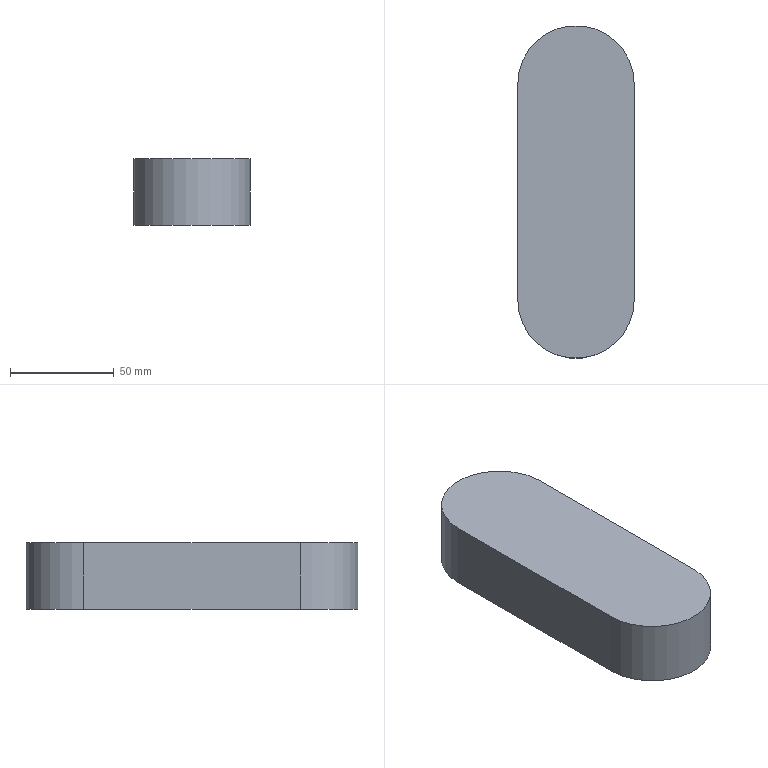Part | SolidWorks | features Extrusion 1 | 1 solid | 6 faces | box 56 x 160 x 32 mm | volume 265184 mm3 | plane 4 | cylinder 2 | commonest cylinder face diameters 56 x2
STEP:
#1=CARTESIAN_POINT('',(0.,0.,0.));
#2=VERTEX_POINT('',#1);
#3=CARTESIAN_POINT('',(0.,104.,0.));
#4=VERTEX_POINT('',#3);
#5=CARTESIAN_POINT('',(0.,0.,0.));
#6=DIRECTION('',(0.,1.,0.));
#7=VECTOR('',#6,1000.);
#8=LINE('',#5,#7);
#9=EDGE_CURVE('',#2,#4,#8,.T.);
#10=ORIENTED_EDGE('',*,*,#9,.F.);
#11=CARTESIAN_POINT('',(0.,0.,32.));
#12=VERTEX_POINT('',#11);
#13=CARTESIAN_POINT('',(0.,0.,32.));
#14=DIRECTION('',(0.,0.,-1.));
#15=VECTOR('',#14,1000.);
#16=LINE('',#13,#15);
#17=EDGE_CURVE('',#12,#2,#16,.T.);
#18=ORIENTED_EDGE('',*,*,#17,.F.);
#19=CARTESIAN_POINT('',(0.,104.,32.));
#20=VERTEX_POINT('',#19);
#21=CARTESIAN_POINT('',(0.,0.,32.));
#22=DIRECTION('',(0.,1.,0.));
#23=VECTOR('',#22,1000.);
#24=LINE('',#21,#23);
#25=EDGE_CURVE('',#12,#20,#24,.T.);
#26=ORIENTED_EDGE('',*,*,#25,.T.);
#27=CARTESIAN_POINT('',(0.,104.,32.));
#28=DIRECTION('',(0.,0.,-1.));
#29=VECTOR('',#28,1000.);
#30=LINE('',#27,#29);
#31=EDGE_CURVE('',#20,#4,#30,.T.);
#32=ORIENTED_EDGE('',*,*,#31,.T.);
#33=EDGE_LOOP('',(#10,#18,#26,#32));
#34=FACE_OUTER_BOUND('',#33,.T.);
#35=CARTESIAN_POINT('',(0.,0.,32.));
#36=DIRECTION('',(-1.,0.,0.));
#37=DIRECTION('',(0.,0.,1.));
#38=AXIS2_PLACEMENT_3D('',#35,#36,#37);
#39=PLANE('',#38);
#40=ADVANCED_FACE('',(#34),#39,.T.);
#41=CARTESIAN_POINT('',(56.,0.,0.));
#42=VERTEX_POINT('',#41);
#43=CARTESIAN_POINT('',(28.,0.,0.));
#44=DIRECTION('',(0.,0.,1.));
#45=DIRECTION('',(1.,0.,0.));
#46=AXIS2_PLACEMENT_3D('',#43,#44,#45);
#47=CIRCLE('',#46,28.);
#48=EDGE_CURVE('',#2,#42,#47,.T.);
#49=ORIENTED_EDGE('',*,*,#48,.T.);
#50=CARTESIAN_POINT('',(56.,0.,32.));
#51=VERTEX_POINT('',#50);
#52=CARTESIAN_POINT('',(56.,0.,32.));
#53=DIRECTION('',(0.,0.,-1.));
#54=VECTOR('',#53,1000.);
#55=LINE('',#52,#54);
#56=EDGE_CURVE('',#51,#42,#55,.T.);
#57=ORIENTED_EDGE('',*,*,#56,.F.);
#58=CARTESIAN_POINT('',(28.,0.,32.));
#59=DIRECTION('',(0.,0.,1.));
#60=DIRECTION('',(1.,0.,0.));
#61=AXIS2_PLACEMENT_3D('',#58,#59,#60);
#62=CIRCLE('',#61,28.);
#63=EDGE_CURVE('',#12,#51,#62,.T.);
#64=ORIENTED_EDGE('',*,*,#63,.F.);
#65=ORIENTED_EDGE('',*,*,#17,.T.);
#66=EDGE_LOOP('',(#49,#57,#64,#65));
#67=FACE_OUTER_BOUND('',#66,.T.);
#68=CARTESIAN_POINT('',(28.,0.,32.));
#69=DIRECTION('',(0.,0.,-1.));
#70=DIRECTION('',(-1.,0.,0.));
#71=AXIS2_PLACEMENT_3D('',#68,#69,#70);
#72=CYLINDRICAL_SURFACE('',#71,28.);
#73=ADVANCED_FACE('',(#67),#72,.T.);
#74=CARTESIAN_POINT('',(56.,104.,0.));
#75=VERTEX_POINT('',#74);
#76=CARTESIAN_POINT('',(56.,0.,0.));
#77=DIRECTION('',(0.,-1.,0.));
#78=VECTOR('',#77,1000.);
#79=LINE('',#76,#78);
#80=EDGE_CURVE('',#75,#42,#79,.T.);
#81=ORIENTED_EDGE('',*,*,#80,.F.);
#82=CARTESIAN_POINT('',(56.,104.,32.));
#83=VERTEX_POINT('',#82);
#84=CARTESIAN_POINT('',(56.,104.,32.));
#85=DIRECTION('',(0.,0.,-1.));
#86=VECTOR('',#85,1000.);
#87=LINE('',#84,#86);
#88=EDGE_CURVE('',#83,#75,#87,.T.);
#89=ORIENTED_EDGE('',*,*,#88,.F.);
#90=CARTESIAN_POINT('',(56.,0.,32.));
#91=DIRECTION('',(0.,-1.,0.));
#92=VECTOR('',#91,1000.);
#93=LINE('',#90,#92);
#94=EDGE_CURVE('',#83,#51,#93,.T.);
#95=ORIENTED_EDGE('',*,*,#94,.T.);
#96=ORIENTED_EDGE('',*,*,#56,.T.);
#97=EDGE_LOOP('',(#81,#89,#95,#96));
#98=FACE_OUTER_BOUND('',#97,.T.);
#99=CARTESIAN_POINT('',(56.,0.,32.));
#100=DIRECTION('',(1.,0.,0.));
#101=DIRECTION('',(0.,0.,-1.));
#102=AXIS2_PLACEMENT_3D('',#99,#100,#101);
#103=PLANE('',#102);
#104=ADVANCED_FACE('',(#98),#103,.T.);
#105=CARTESIAN_POINT('',(28.,104.,0.));
#106=DIRECTION('',(0.,0.,-1.));
#107=DIRECTION('',(1.,0.,0.));
#108=AXIS2_PLACEMENT_3D('',#105,#106,#107);
#109=CIRCLE('',#108,28.);
#110=EDGE_CURVE('',#4,#75,#109,.T.);
#111=ORIENTED_EDGE('',*,*,#110,.F.);
#112=ORIENTED_EDGE('',*,*,#31,.F.);
#113=CARTESIAN_POINT('',(28.,104.,32.));
#114=DIRECTION('',(0.,0.,-1.));
#115=DIRECTION('',(1.,0.,0.));
#116=AXIS2_PLACEMENT_3D('',#113,#114,#115);
#117=CIRCLE('',#116,28.);
#118=EDGE_CURVE('',#20,#83,#117,.T.);
#119=ORIENTED_EDGE('',*,*,#118,.T.);
#120=ORIENTED_EDGE('',*,*,#88,.T.);
#121=EDGE_LOOP('',(#111,#112,#119,#120));
#122=FACE_OUTER_BOUND('',#121,.T.);
#123=CARTESIAN_POINT('',(28.,104.,32.));
#124=DIRECTION('',(0.,0.,-1.));
#125=DIRECTION('',(-1.,0.,0.));
#126=AXIS2_PLACEMENT_3D('',#123,#124,#125);
#127=CYLINDRICAL_SURFACE('',#126,28.);
#128=ADVANCED_FACE('',(#122),#127,.T.);
#129=ORIENTED_EDGE('',*,*,#25,.F.);
#130=ORIENTED_EDGE('',*,*,#63,.T.);
#131=ORIENTED_EDGE('',*,*,#94,.F.);
#132=ORIENTED_EDGE('',*,*,#118,.F.);
#133=EDGE_LOOP('',(#129,#130,#131,#132));
#134=FACE_OUTER_BOUND('',#133,.T.);
#135=CARTESIAN_POINT('',(0.,0.,32.));
#136=DIRECTION('',(0.,0.,1.));
#137=DIRECTION('',(1.,0.,0.));
#138=AXIS2_PLACEMENT_3D('',#135,#136,#137);
#139=PLANE('',#138);
#140=ADVANCED_FACE('',(#134),#139,.T.);
#141=ORIENTED_EDGE('',*,*,#9,.T.);
#142=ORIENTED_EDGE('',*,*,#110,.T.);
#143=ORIENTED_EDGE('',*,*,#80,.T.);
#144=ORIENTED_EDGE('',*,*,#48,.F.);
#145=EDGE_LOOP('',(#141,#142,#143,#144));
#146=FACE_OUTER_BOUND('',#145,.T.);
#147=CARTESIAN_POINT('',(0.,0.,0.));
#148=DIRECTION('',(0.,0.,1.));
#149=DIRECTION('',(1.,0.,0.));
#150=AXIS2_PLACEMENT_3D('',#147,#148,#149);
#151=PLANE('',#150);
#152=ADVANCED_FACE('',(#146),#151,.F.);
#153=CLOSED_SHELL('',(#40,#73,#104,#128,#140,#152));
#154=MANIFOLD_SOLID_BREP('',#153);
#155=CARTESIAN_POINT('',(0.,0.,0.));
#156=DIRECTION('',(0.,0.,1.));
#157=DIRECTION('',(1.,0.,0.));
#158=AXIS2_PLACEMENT_3D('',#155,#156,#157);
#159=(LENGTH_UNIT()NAMED_UNIT(*)SI_UNIT(.MILLI.,.METRE.));
#160=UNCERTAINTY_MEASURE_WITH_UNIT(LENGTH_MEASURE(0.00001),#159,'','');
#161=(NAMED_UNIT(*)PLANE_ANGLE_UNIT()SI_UNIT($,.RADIAN.));
#162=(NAMED_UNIT(*)SI_UNIT($,.STERADIAN.)SOLID_ANGLE_UNIT());
#163=(GEOMETRIC_REPRESENTATION_CONTEXT(3)GLOBAL_UNCERTAINTY_ASSIGNED_CONTEXT((#160))GLOBAL_UNIT_ASSIGNED_CONTEXT((#159,#161,#162))REPRESENTATION_CONTEXT('',''));
#164=ADVANCED_BREP_SHAPE_REPRESENTATION('',(#154,#158),#163);